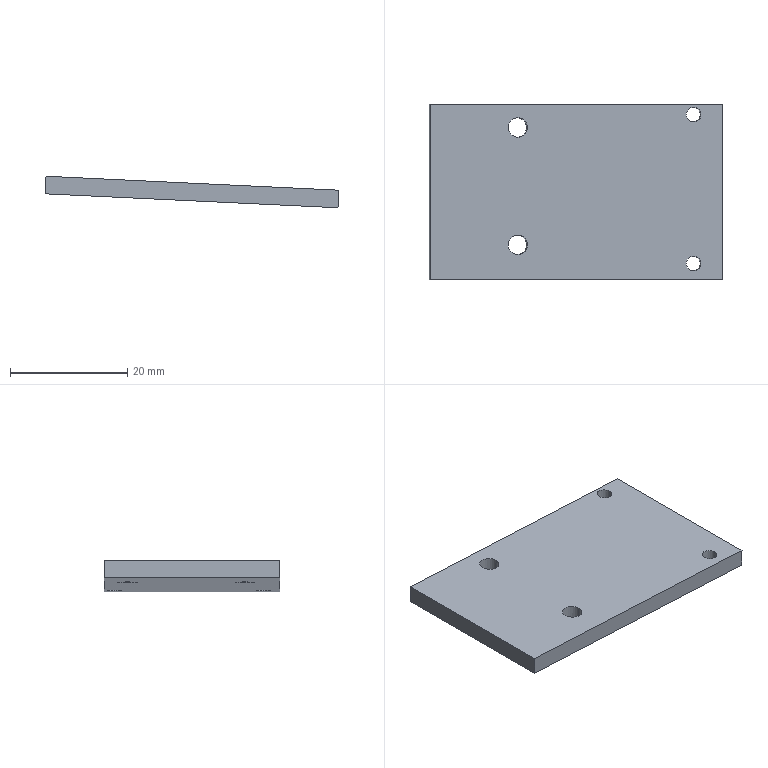Part | SolidWorks | features HoleWzd 2, Extrusion 1 | 1 solid | 14 faces | box 50.086 x 30 x 5.375 mm | volume 4419 mm3 | cylinder 8 | plane 6 | commonest cylinder face diameters 2.5 x4 3.3 x4
STEP:
#1=CARTESIAN_POINT('',(32.309,322.2,1.906));
#2=VERTEX_POINT('',#1);
#3=CARTESIAN_POINT('',(29.811,322.2,2.025));
#4=VERTEX_POINT('',#3);
#5=CARTESIAN_POINT('',(31.06,322.2,1.966));
#6=DIRECTION('',(-0.04757,0.,-0.9989));
#7=DIRECTION('',(-0.9989,0.,0.04757));
#8=AXIS2_PLACEMENT_3D('',#5,#6,#7);
#9=CIRCLE('',#8,1.25);
#10=EDGE_CURVE('',#2,#4,#9,.T.);
#11=ORIENTED_EDGE('',*,*,#10,.F.);
#12=CARTESIAN_POINT('',(32.166,322.2,-1.09));
#13=VERTEX_POINT('',#12);
#14=CARTESIAN_POINT('',(32.166,322.2,-1.09));
#15=DIRECTION('',(-0.04757,0.,-0.9989));
#16=VECTOR('',#15,1000.);
#17=LINE('',#14,#16);
#18=EDGE_CURVE('',#2,#13,#17,.T.);
#19=ORIENTED_EDGE('',*,*,#18,.T.);
#20=CARTESIAN_POINT('',(29.669,322.2,-0.9715));
#21=VERTEX_POINT('',#20);
#22=CARTESIAN_POINT('',(30.917,322.2,-1.031));
#23=DIRECTION('',(-0.04757,0.,-0.9989));
#24=DIRECTION('',(-0.9989,0.,0.04757));
#25=AXIS2_PLACEMENT_3D('',#22,#23,#24);
#26=CIRCLE('',#25,1.25);
#27=EDGE_CURVE('',#13,#21,#26,.T.);
#28=ORIENTED_EDGE('',*,*,#27,.T.);
#29=CARTESIAN_POINT('',(29.669,322.2,-0.9715));
#30=DIRECTION('',(-0.04757,0.,-0.9989));
#31=VECTOR('',#30,1000.);
#32=LINE('',#29,#31);
#33=EDGE_CURVE('',#4,#21,#32,.T.);
#34=ORIENTED_EDGE('',*,*,#33,.F.);
#35=EDGE_LOOP('',(#11,#19,#28,#34));
#36=FACE_OUTER_BOUND('',#35,.T.);
#37=CARTESIAN_POINT('',(30.917,322.2,-1.031));
#38=DIRECTION('',(-0.04757,0.,-0.9989));
#39=DIRECTION('',(-0.9989,0.,0.04757));
#40=AXIS2_PLACEMENT_3D('',#37,#38,#39);
#41=CYLINDRICAL_SURFACE('',#40,1.25);
#42=ADVANCED_FACE('',(#36),#41,.F.);
#43=CARTESIAN_POINT('',(32.309,296.8,1.906));
#44=VERTEX_POINT('',#43);
#45=CARTESIAN_POINT('',(29.811,296.8,2.025));
#46=VERTEX_POINT('',#45);
#47=CARTESIAN_POINT('',(31.06,296.8,1.966));
#48=DIRECTION('',(-0.04757,0.,-0.9989));
#49=DIRECTION('',(-0.9989,0.,0.04757));
#50=AXIS2_PLACEMENT_3D('',#47,#48,#49);
#51=CIRCLE('',#50,1.25);
#52=EDGE_CURVE('',#44,#46,#51,.T.);
#53=ORIENTED_EDGE('',*,*,#52,.F.);
#54=CARTESIAN_POINT('',(32.166,296.8,-1.09));
#55=VERTEX_POINT('',#54);
#56=CARTESIAN_POINT('',(32.166,296.8,-1.09));
#57=DIRECTION('',(-0.04757,0.,-0.9989));
#58=VECTOR('',#57,1000.);
#59=LINE('',#56,#58);
#60=EDGE_CURVE('',#44,#55,#59,.T.);
#61=ORIENTED_EDGE('',*,*,#60,.T.);
#62=CARTESIAN_POINT('',(29.669,296.8,-0.9715));
#63=VERTEX_POINT('',#62);
#64=CARTESIAN_POINT('',(30.917,296.8,-1.031));
#65=DIRECTION('',(-0.04757,0.,-0.9989));
#66=DIRECTION('',(-0.9989,0.,0.04757));
#67=AXIS2_PLACEMENT_3D('',#64,#65,#66);
#68=CIRCLE('',#67,1.25);
#69=EDGE_CURVE('',#55,#63,#68,.T.);
#70=ORIENTED_EDGE('',*,*,#69,.T.);
#71=CARTESIAN_POINT('',(29.669,296.8,-0.9715));
#72=DIRECTION('',(-0.04757,0.,-0.9989));
#73=VECTOR('',#72,1000.);
#74=LINE('',#71,#73);
#75=EDGE_CURVE('',#46,#63,#74,.T.);
#76=ORIENTED_EDGE('',*,*,#75,.F.);
#77=EDGE_LOOP('',(#53,#61,#70,#76));
#78=FACE_OUTER_BOUND('',#77,.T.);
#79=CARTESIAN_POINT('',(30.917,296.8,-1.031));
#80=DIRECTION('',(-0.04757,0.,-0.9989));
#81=DIRECTION('',(-0.9989,0.,0.04757));
#82=AXIS2_PLACEMENT_3D('',#79,#80,#81);
#83=CYLINDRICAL_SURFACE('',#82,1.25);
#84=ADVANCED_FACE('',(#78),#83,.F.);
#85=CARTESIAN_POINT('',(2.742,320.,3.314));
#86=VERTEX_POINT('',#85);
#87=CARTESIAN_POINT('',(-0.5541,320.,3.471));
#88=VERTEX_POINT('',#87);
#89=CARTESIAN_POINT('',(1.094,320.,3.393));
#90=DIRECTION('',(-0.04757,0.,-0.9989));
#91=DIRECTION('',(-0.9989,0.,0.04757));
#92=AXIS2_PLACEMENT_3D('',#89,#90,#91);
#93=CIRCLE('',#92,1.65);
#94=EDGE_CURVE('',#86,#88,#93,.T.);
#95=ORIENTED_EDGE('',*,*,#94,.F.);
#96=CARTESIAN_POINT('',(2.599,320.,0.3175));
#97=VERTEX_POINT('',#96);
#98=CARTESIAN_POINT('',(2.599,320.,0.3175));
#99=DIRECTION('',(-0.04757,0.,-0.9989));
#100=VECTOR('',#99,1000.);
#101=LINE('',#98,#100);
#102=EDGE_CURVE('',#86,#97,#101,.T.);
#103=ORIENTED_EDGE('',*,*,#102,.T.);
#104=CARTESIAN_POINT('',(-0.6968,320.,0.4745));
#105=VERTEX_POINT('',#104);
#106=CARTESIAN_POINT('',(0.9513,320.,0.396));
#107=DIRECTION('',(-0.04757,0.,-0.9989));
#108=DIRECTION('',(-0.9989,0.,0.04757));
#109=AXIS2_PLACEMENT_3D('',#106,#107,#108);
#110=CIRCLE('',#109,1.65);
#111=EDGE_CURVE('',#97,#105,#110,.T.);
#112=ORIENTED_EDGE('',*,*,#111,.T.);
#113=CARTESIAN_POINT('',(-0.6968,320.,0.4745));
#114=DIRECTION('',(-0.04757,0.,-0.9989));
#115=VECTOR('',#114,1000.);
#116=LINE('',#113,#115);
#117=EDGE_CURVE('',#88,#105,#116,.T.);
#118=ORIENTED_EDGE('',*,*,#117,.F.);
#119=EDGE_LOOP('',(#95,#103,#112,#118));
#120=FACE_OUTER_BOUND('',#119,.T.);
#121=CARTESIAN_POINT('',(0.9513,320.,0.396));
#122=DIRECTION('',(-0.04757,0.,-0.9989));
#123=DIRECTION('',(-0.9989,0.,0.04757));
#124=AXIS2_PLACEMENT_3D('',#121,#122,#123);
#125=CYLINDRICAL_SURFACE('',#124,1.65);
#126=ADVANCED_FACE('',(#120),#125,.F.);
#127=CARTESIAN_POINT('',(2.742,300.,3.314));
#128=VERTEX_POINT('',#127);
#129=CARTESIAN_POINT('',(-0.5541,300.,3.471));
#130=VERTEX_POINT('',#129);
#131=CARTESIAN_POINT('',(1.094,300.,3.393));
#132=DIRECTION('',(-0.04757,0.,-0.9989));
#133=DIRECTION('',(-0.9989,0.,0.04757));
#134=AXIS2_PLACEMENT_3D('',#131,#132,#133);
#135=CIRCLE('',#134,1.65);
#136=EDGE_CURVE('',#128,#130,#135,.T.);
#137=ORIENTED_EDGE('',*,*,#136,.F.);
#138=CARTESIAN_POINT('',(2.599,300.,0.3175));
#139=VERTEX_POINT('',#138);
#140=CARTESIAN_POINT('',(2.599,300.,0.3175));
#141=DIRECTION('',(-0.04757,0.,-0.9989));
#142=VECTOR('',#141,1000.);
#143=LINE('',#140,#142);
#144=EDGE_CURVE('',#128,#139,#143,.T.);
#145=ORIENTED_EDGE('',*,*,#144,.T.);
#146=CARTESIAN_POINT('',(-0.6968,300.,0.4745));
#147=VERTEX_POINT('',#146);
#148=CARTESIAN_POINT('',(0.9513,300.,0.396));
#149=DIRECTION('',(-0.04757,0.,-0.9989));
#150=DIRECTION('',(-0.9989,0.,0.04757));
#151=AXIS2_PLACEMENT_3D('',#148,#149,#150);
#152=CIRCLE('',#151,1.65);
#153=EDGE_CURVE('',#139,#147,#152,.T.);
#154=ORIENTED_EDGE('',*,*,#153,.T.);
#155=CARTESIAN_POINT('',(-0.6968,300.,0.4745));
#156=DIRECTION('',(-0.04757,0.,-0.9989));
#157=VECTOR('',#156,1000.);
#158=LINE('',#155,#157);
#159=EDGE_CURVE('',#130,#147,#158,.T.);
#160=ORIENTED_EDGE('',*,*,#159,.F.);
#161=EDGE_LOOP('',(#137,#145,#154,#160));
#162=FACE_OUTER_BOUND('',#161,.T.);
#163=CARTESIAN_POINT('',(0.9513,300.,0.396));
#164=DIRECTION('',(-0.04757,0.,-0.9989));
#165=DIRECTION('',(-0.9989,0.,0.04757));
#166=AXIS2_PLACEMENT_3D('',#163,#164,#165);
#167=CYLINDRICAL_SURFACE('',#166,1.65);
#168=ADVANCED_FACE('',(#162),#167,.F.);
#169=CARTESIAN_POINT('',(35.912,324.,-1.269));
#170=VERTEX_POINT('',#169);
#171=CARTESIAN_POINT('',(35.912,294.,-1.269));
#172=VERTEX_POINT('',#171);
#173=CARTESIAN_POINT('',(35.912,324.,-1.269));
#174=DIRECTION('',(0.,-1.,0.));
#175=VECTOR('',#174,1000.);
#176=LINE('',#173,#175);
#177=EDGE_CURVE('',#170,#172,#176,.T.);
#178=ORIENTED_EDGE('',*,*,#177,.F.);
#179=CARTESIAN_POINT('',(36.054,324.,1.728));
#180=VERTEX_POINT('',#179);
#181=CARTESIAN_POINT('',(36.054,324.,1.728));
#182=DIRECTION('',(-0.04757,0.,-0.9989));
#183=VECTOR('',#182,1000.);
#184=LINE('',#181,#183);
#185=EDGE_CURVE('',#180,#170,#184,.T.);
#186=ORIENTED_EDGE('',*,*,#185,.F.);
#187=CARTESIAN_POINT('',(36.054,294.,1.728));
#188=VERTEX_POINT('',#187);
#189=CARTESIAN_POINT('',(36.054,324.,1.728));
#190=DIRECTION('',(0.,-1.,0.));
#191=VECTOR('',#190,1000.);
#192=LINE('',#189,#191);
#193=EDGE_CURVE('',#180,#188,#192,.T.);
#194=ORIENTED_EDGE('',*,*,#193,.T.);
#195=CARTESIAN_POINT('',(36.054,294.,1.728));
#196=DIRECTION('',(-0.04757,0.,-0.9989));
#197=VECTOR('',#196,1000.);
#198=LINE('',#195,#197);
#199=EDGE_CURVE('',#188,#172,#198,.T.);
#200=ORIENTED_EDGE('',*,*,#199,.T.);
#201=EDGE_LOOP('',(#178,#186,#194,#200));
#202=FACE_OUTER_BOUND('',#201,.T.);
#203=CARTESIAN_POINT('',(36.054,324.,1.728));
#204=DIRECTION('',(0.9989,0.,-0.04757));
#205=DIRECTION('',(-0.04757,0.,-0.9989));
#206=AXIS2_PLACEMENT_3D('',#203,#204,#205);
#207=PLANE('',#206);
#208=ADVANCED_FACE('',(#202),#207,.T.);
#209=CARTESIAN_POINT('',(-14.032,324.,1.109));
#210=VERTEX_POINT('',#209);
#211=CARTESIAN_POINT('',(35.912,324.,-1.269));
#212=DIRECTION('',(-0.9989,0.,0.04757));
#213=VECTOR('',#212,1000.);
#214=LINE('',#211,#213);
#215=EDGE_CURVE('',#170,#210,#214,.T.);
#216=ORIENTED_EDGE('',*,*,#215,.T.);
#217=CARTESIAN_POINT('',(-13.889,324.,4.106));
#218=VERTEX_POINT('',#217);
#219=CARTESIAN_POINT('',(-13.889,324.,4.106));
#220=DIRECTION('',(-0.04757,0.,-0.9989));
#221=VECTOR('',#220,1000.);
#222=LINE('',#219,#221);
#223=EDGE_CURVE('',#218,#210,#222,.T.);
#224=ORIENTED_EDGE('',*,*,#223,.F.);
#225=CARTESIAN_POINT('',(36.054,324.,1.728));
#226=DIRECTION('',(-0.9989,0.,0.04757));
#227=VECTOR('',#226,1000.);
#228=LINE('',#225,#227);
#229=EDGE_CURVE('',#180,#218,#228,.T.);
#230=ORIENTED_EDGE('',*,*,#229,.F.);
#231=ORIENTED_EDGE('',*,*,#185,.T.);
#232=EDGE_LOOP('',(#216,#224,#230,#231));
#233=FACE_OUTER_BOUND('',#232,.T.);
#234=CARTESIAN_POINT('',(36.054,324.,1.728));
#235=DIRECTION('',(0.,-1.,0.));
#236=DIRECTION('',(0.,0.,-1.));
#237=AXIS2_PLACEMENT_3D('',#234,#235,#236);
#238=PLANE('',#237);
#239=ADVANCED_FACE('',(#233),#238,.F.);
#240=CARTESIAN_POINT('',(-14.032,294.,1.109));
#241=VERTEX_POINT('',#240);
#242=CARTESIAN_POINT('',(-14.032,324.,1.109));
#243=DIRECTION('',(0.,-1.,0.));
#244=VECTOR('',#243,1000.);
#245=LINE('',#242,#244);
#246=EDGE_CURVE('',#210,#241,#245,.T.);
#247=ORIENTED_EDGE('',*,*,#246,.T.);
#248=CARTESIAN_POINT('',(-13.889,294.,4.106));
#249=VERTEX_POINT('',#248);
#250=CARTESIAN_POINT('',(-13.889,294.,4.106));
#251=DIRECTION('',(-0.04757,0.,-0.9989));
#252=VECTOR('',#251,1000.);
#253=LINE('',#250,#252);
#254=EDGE_CURVE('',#249,#241,#253,.T.);
#255=ORIENTED_EDGE('',*,*,#254,.F.);
#256=CARTESIAN_POINT('',(-13.889,324.,4.106));
#257=DIRECTION('',(0.,-1.,0.));
#258=VECTOR('',#257,1000.);
#259=LINE('',#256,#258);
#260=EDGE_CURVE('',#218,#249,#259,.T.);
#261=ORIENTED_EDGE('',*,*,#260,.F.);
#262=ORIENTED_EDGE('',*,*,#223,.T.);
#263=EDGE_LOOP('',(#247,#255,#261,#262));
#264=FACE_OUTER_BOUND('',#263,.T.);
#265=CARTESIAN_POINT('',(-13.889,324.,4.106));
#266=DIRECTION('',(0.9989,0.,-0.04757));
#267=DIRECTION('',(-0.04757,0.,-0.9989));
#268=AXIS2_PLACEMENT_3D('',#265,#266,#267);
#269=PLANE('',#268);
#270=ADVANCED_FACE('',(#264),#269,.F.);
#271=CARTESIAN_POINT('',(35.912,294.,-1.269));
#272=DIRECTION('',(-0.9989,0.,0.04757));
#273=VECTOR('',#272,1000.);
#274=LINE('',#271,#273);
#275=EDGE_CURVE('',#172,#241,#274,.T.);
#276=ORIENTED_EDGE('',*,*,#275,.F.);
#277=ORIENTED_EDGE('',*,*,#199,.F.);
#278=CARTESIAN_POINT('',(36.054,294.,1.728));
#279=DIRECTION('',(-0.9989,0.,0.04757));
#280=VECTOR('',#279,1000.);
#281=LINE('',#278,#280);
#282=EDGE_CURVE('',#188,#249,#281,.T.);
#283=ORIENTED_EDGE('',*,*,#282,.T.);
#284=ORIENTED_EDGE('',*,*,#254,.T.);
#285=EDGE_LOOP('',(#276,#277,#283,#284));
#286=FACE_OUTER_BOUND('',#285,.T.);
#287=CARTESIAN_POINT('',(36.054,294.,1.728));
#288=DIRECTION('',(0.,-1.,0.));
#289=DIRECTION('',(1.,0.,0.));
#290=AXIS2_PLACEMENT_3D('',#287,#288,#289);
#291=PLANE('',#290);
#292=ADVANCED_FACE('',(#286),#291,.T.);
#293=CARTESIAN_POINT('',(31.06,322.2,1.966));
#294=DIRECTION('',(-0.04757,0.,-0.9989));
#295=DIRECTION('',(-0.9989,0.,0.04757));
#296=AXIS2_PLACEMENT_3D('',#293,#294,#295);
#297=CIRCLE('',#296,1.25);
#298=EDGE_CURVE('',#4,#2,#297,.T.);
#299=ORIENTED_EDGE('',*,*,#298,.T.);
#300=ORIENTED_EDGE('',*,*,#10,.T.);
#301=EDGE_LOOP('',(#299,#300));
#302=FACE_BOUND('',#301,.T.);
#303=CARTESIAN_POINT('',(31.06,296.8,1.966));
#304=DIRECTION('',(-0.04757,0.,-0.9989));
#305=DIRECTION('',(-0.9989,0.,0.04757));
#306=AXIS2_PLACEMENT_3D('',#303,#304,#305);
#307=CIRCLE('',#306,1.25);
#308=EDGE_CURVE('',#46,#44,#307,.T.);
#309=ORIENTED_EDGE('',*,*,#308,.T.);
#310=ORIENTED_EDGE('',*,*,#52,.T.);
#311=EDGE_LOOP('',(#309,#310));
#312=FACE_BOUND('',#311,.T.);
#313=CARTESIAN_POINT('',(1.094,320.,3.393));
#314=DIRECTION('',(-0.04757,0.,-0.9989));
#315=DIRECTION('',(-0.9989,0.,0.04757));
#316=AXIS2_PLACEMENT_3D('',#313,#314,#315);
#317=CIRCLE('',#316,1.65);
#318=EDGE_CURVE('',#88,#86,#317,.T.);
#319=ORIENTED_EDGE('',*,*,#318,.T.);
#320=ORIENTED_EDGE('',*,*,#94,.T.);
#321=EDGE_LOOP('',(#319,#320));
#322=FACE_BOUND('',#321,.T.);
#323=CARTESIAN_POINT('',(1.094,300.,3.393));
#324=DIRECTION('',(-0.04757,0.,-0.9989));
#325=DIRECTION('',(-0.9989,0.,0.04757));
#326=AXIS2_PLACEMENT_3D('',#323,#324,#325);
#327=CIRCLE('',#326,1.65);
#328=EDGE_CURVE('',#130,#128,#327,.T.);
#329=ORIENTED_EDGE('',*,*,#328,.T.);
#330=ORIENTED_EDGE('',*,*,#136,.T.);
#331=EDGE_LOOP('',(#329,#330));
#332=FACE_BOUND('',#331,.T.);
#333=ORIENTED_EDGE('',*,*,#193,.F.);
#334=ORIENTED_EDGE('',*,*,#229,.T.);
#335=ORIENTED_EDGE('',*,*,#260,.T.);
#336=ORIENTED_EDGE('',*,*,#282,.F.);
#337=EDGE_LOOP('',(#333,#334,#335,#336));
#338=FACE_OUTER_BOUND('',#337,.T.);
#339=CARTESIAN_POINT('',(0.1637,0.,3.437));
#340=DIRECTION('',(-0.04757,0.,-0.9989));
#341=DIRECTION('',(-0.9989,0.,0.04757));
#342=AXIS2_PLACEMENT_3D('',#339,#340,#341);
#343=PLANE('',#342);
#344=ADVANCED_FACE('',(#302,#312,#322,#332,#338),#343,.F.);
#345=CARTESIAN_POINT('',(30.917,322.2,-1.031));
#346=DIRECTION('',(-0.04757,0.,-0.9989));
#347=DIRECTION('',(-0.9989,0.,0.04757));
#348=AXIS2_PLACEMENT_3D('',#345,#346,#347);
#349=CIRCLE('',#348,1.25);
#350=EDGE_CURVE('',#21,#13,#349,.T.);
#351=ORIENTED_EDGE('',*,*,#350,.F.);
#352=ORIENTED_EDGE('',*,*,#27,.F.);
#353=EDGE_LOOP('',(#351,#352));
#354=FACE_BOUND('',#353,.T.);
#355=CARTESIAN_POINT('',(30.917,296.8,-1.031));
#356=DIRECTION('',(-0.04757,0.,-0.9989));
#357=DIRECTION('',(-0.9989,0.,0.04757));
#358=AXIS2_PLACEMENT_3D('',#355,#356,#357);
#359=CIRCLE('',#358,1.25);
#360=EDGE_CURVE('',#63,#55,#359,.T.);
#361=ORIENTED_EDGE('',*,*,#360,.F.);
#362=ORIENTED_EDGE('',*,*,#69,.F.);
#363=EDGE_LOOP('',(#361,#362));
#364=FACE_BOUND('',#363,.T.);
#365=CARTESIAN_POINT('',(0.9513,320.,0.396));
#366=DIRECTION('',(-0.04757,0.,-0.9989));
#367=DIRECTION('',(-0.9989,0.,0.04757));
#368=AXIS2_PLACEMENT_3D('',#365,#366,#367);
#369=CIRCLE('',#368,1.65);
#370=EDGE_CURVE('',#105,#97,#369,.T.);
#371=ORIENTED_EDGE('',*,*,#370,.F.);
#372=ORIENTED_EDGE('',*,*,#111,.F.);
#373=EDGE_LOOP('',(#371,#372));
#374=FACE_BOUND('',#373,.T.);
#375=CARTESIAN_POINT('',(0.9513,300.,0.396));
#376=DIRECTION('',(-0.04757,0.,-0.9989));
#377=DIRECTION('',(-0.9989,0.,0.04757));
#378=AXIS2_PLACEMENT_3D('',#375,#376,#377);
#379=CIRCLE('',#378,1.65);
#380=EDGE_CURVE('',#147,#139,#379,.T.);
#381=ORIENTED_EDGE('',*,*,#380,.F.);
#382=ORIENTED_EDGE('',*,*,#153,.F.);
#383=EDGE_LOOP('',(#381,#382));
#384=FACE_BOUND('',#383,.T.);
#385=ORIENTED_EDGE('',*,*,#177,.T.);
#386=ORIENTED_EDGE('',*,*,#275,.T.);
#387=ORIENTED_EDGE('',*,*,#246,.F.);
#388=ORIENTED_EDGE('',*,*,#215,.F.);
#389=EDGE_LOOP('',(#385,#386,#387,#388));
#390=FACE_OUTER_BOUND('',#389,.T.);
#391=CARTESIAN_POINT('',(0.02097,0.,0.4403));
#392=DIRECTION('',(-0.04757,0.,-0.9989));
#393=DIRECTION('',(-0.9989,0.,0.04757));
#394=AXIS2_PLACEMENT_3D('',#391,#392,#393);
#395=PLANE('',#394);
#396=ADVANCED_FACE('',(#354,#364,#374,#384,#390),#395,.T.);
#397=ORIENTED_EDGE('',*,*,#144,.F.);
#398=ORIENTED_EDGE('',*,*,#328,.F.);
#399=ORIENTED_EDGE('',*,*,#159,.T.);
#400=ORIENTED_EDGE('',*,*,#380,.T.);
#401=EDGE_LOOP('',(#397,#398,#399,#400));
#402=FACE_OUTER_BOUND('',#401,.T.);
#403=CARTESIAN_POINT('',(0.9513,300.,0.396));
#404=DIRECTION('',(-0.04757,0.,-0.9989));
#405=DIRECTION('',(-0.9989,0.,0.04757));
#406=AXIS2_PLACEMENT_3D('',#403,#404,#405);
#407=CYLINDRICAL_SURFACE('',#406,1.65);
#408=ADVANCED_FACE('',(#402),#407,.F.);
#409=ORIENTED_EDGE('',*,*,#102,.F.);
#410=ORIENTED_EDGE('',*,*,#318,.F.);
#411=ORIENTED_EDGE('',*,*,#117,.T.);
#412=ORIENTED_EDGE('',*,*,#370,.T.);
#413=EDGE_LOOP('',(#409,#410,#411,#412));
#414=FACE_OUTER_BOUND('',#413,.T.);
#415=CARTESIAN_POINT('',(0.9513,320.,0.396));
#416=DIRECTION('',(-0.04757,0.,-0.9989));
#417=DIRECTION('',(-0.9989,0.,0.04757));
#418=AXIS2_PLACEMENT_3D('',#415,#416,#417);
#419=CYLINDRICAL_SURFACE('',#418,1.65);
#420=ADVANCED_FACE('',(#414),#419,.F.);
#421=ORIENTED_EDGE('',*,*,#60,.F.);
#422=ORIENTED_EDGE('',*,*,#308,.F.);
#423=ORIENTED_EDGE('',*,*,#75,.T.);
#424=ORIENTED_EDGE('',*,*,#360,.T.);
#425=EDGE_LOOP('',(#421,#422,#423,#424));
#426=FACE_OUTER_BOUND('',#425,.T.);
#427=CARTESIAN_POINT('',(30.917,296.8,-1.031));
#428=DIRECTION('',(-0.04757,0.,-0.9989));
#429=DIRECTION('',(-0.9989,0.,0.04757));
#430=AXIS2_PLACEMENT_3D('',#427,#428,#429);
#431=CYLINDRICAL_SURFACE('',#430,1.25);
#432=ADVANCED_FACE('',(#426),#431,.F.);
#433=ORIENTED_EDGE('',*,*,#18,.F.);
#434=ORIENTED_EDGE('',*,*,#298,.F.);
#435=ORIENTED_EDGE('',*,*,#33,.T.);
#436=ORIENTED_EDGE('',*,*,#350,.T.);
#437=EDGE_LOOP('',(#433,#434,#435,#436));
#438=FACE_OUTER_BOUND('',#437,.T.);
#439=CARTESIAN_POINT('',(30.917,322.2,-1.031));
#440=DIRECTION('',(-0.04757,0.,-0.9989));
#441=DIRECTION('',(-0.9989,0.,0.04757));
#442=AXIS2_PLACEMENT_3D('',#439,#440,#441);
#443=CYLINDRICAL_SURFACE('',#442,1.25);
#444=ADVANCED_FACE('',(#438),#443,.F.);
#445=CLOSED_SHELL('',(#42,#84,#126,#168,#208,#239,#270,#292,#344,#396,#408,#420,#432,#444));
#446=MANIFOLD_SOLID_BREP('',#445);
#447=CARTESIAN_POINT('',(0.,0.,0.));
#448=DIRECTION('',(0.,0.,1.));
#449=DIRECTION('',(1.,0.,0.));
#450=AXIS2_PLACEMENT_3D('',#447,#448,#449);
#451=(LENGTH_UNIT()NAMED_UNIT(*)SI_UNIT(.MILLI.,.METRE.));
#452=UNCERTAINTY_MEASURE_WITH_UNIT(LENGTH_MEASURE(0.00001),#451,'','');
#453=(NAMED_UNIT(*)PLANE_ANGLE_UNIT()SI_UNIT($,.RADIAN.));
#454=(NAMED_UNIT(*)SI_UNIT($,.STERADIAN.)SOLID_ANGLE_UNIT());
#455=(GEOMETRIC_REPRESENTATION_CONTEXT(3)GLOBAL_UNCERTAINTY_ASSIGNED_CONTEXT((#452))GLOBAL_UNIT_ASSIGNED_CONTEXT((#451,#453,#454))REPRESENTATION_CONTEXT('',''));
#456=ADVANCED_BREP_SHAPE_REPRESENTATION('',(#446,#450),#455);